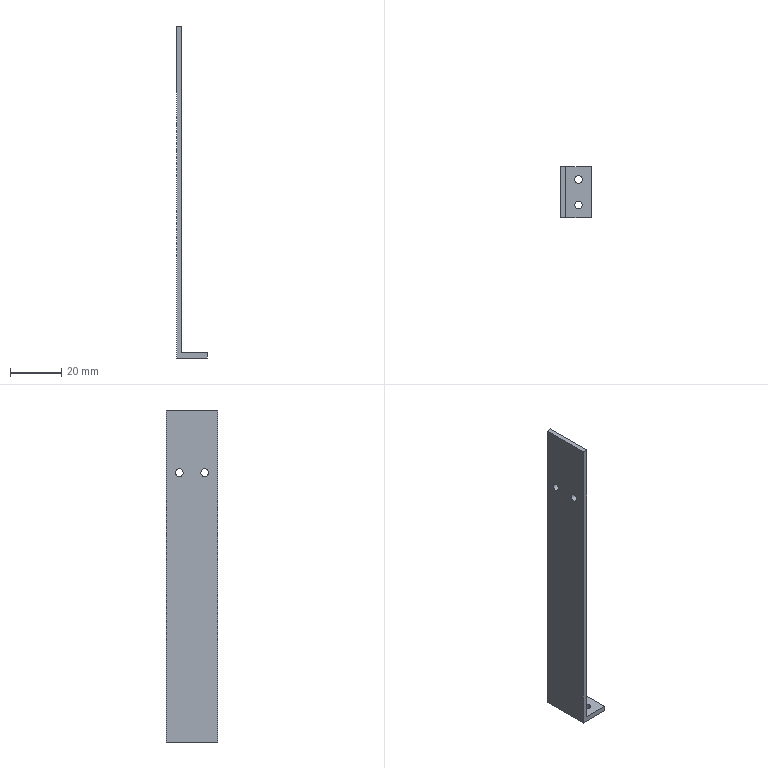Part | SolidWorks | features Cut 2, Extrusion 1, ICE 1 | 1 solid | 16 faces | box 12 x 20 x 130 mm | volume 5543 mm3 | cylinder 8 | plane 8 | commonest cylinder face diameters 3 x8
STEP:
#1=CARTESIAN_POINT('',(10.,-5.,106.942));
#2=VERTEX_POINT('',#1);
#3=CARTESIAN_POINT('',(10.,-5.,103.942));
#4=VERTEX_POINT('',#3);
#5=CARTESIAN_POINT('',(10.,-5.,105.442));
#6=DIRECTION('',(1.,0.,0.));
#7=DIRECTION('',(0.,0.,-1.));
#8=AXIS2_PLACEMENT_3D('',#5,#6,#7);
#9=CIRCLE('',#8,1.5);
#10=EDGE_CURVE('',#2,#4,#9,.T.);
#11=ORIENTED_EDGE('',*,*,#10,.F.);
#12=CARTESIAN_POINT('',(12.,-5.,106.942));
#13=VERTEX_POINT('',#12);
#14=CARTESIAN_POINT('',(-33.,-5.,106.942));
#15=DIRECTION('',(1.,0.,0.));
#16=VECTOR('',#15,1000.);
#17=LINE('',#14,#16);
#18=EDGE_CURVE('',#2,#13,#17,.T.);
#19=ORIENTED_EDGE('',*,*,#18,.T.);
#20=CARTESIAN_POINT('',(12.,-5.,103.942));
#21=VERTEX_POINT('',#20);
#22=CARTESIAN_POINT('',(12.,-5.,105.442));
#23=DIRECTION('',(1.,0.,0.));
#24=DIRECTION('',(0.,0.,-1.));
#25=AXIS2_PLACEMENT_3D('',#22,#23,#24);
#26=CIRCLE('',#25,1.5);
#27=EDGE_CURVE('',#13,#21,#26,.T.);
#28=ORIENTED_EDGE('',*,*,#27,.T.);
#29=CARTESIAN_POINT('',(-33.,-5.,103.942));
#30=DIRECTION('',(1.,0.,0.));
#31=VECTOR('',#30,1000.);
#32=LINE('',#29,#31);
#33=EDGE_CURVE('',#4,#21,#32,.T.);
#34=ORIENTED_EDGE('',*,*,#33,.F.);
#35=EDGE_LOOP('',(#11,#19,#28,#34));
#36=FACE_OUTER_BOUND('',#35,.T.);
#37=CARTESIAN_POINT('',(-33.,-5.,105.442));
#38=DIRECTION('',(1.,0.,0.));
#39=DIRECTION('',(0.,0.,-1.));
#40=AXIS2_PLACEMENT_3D('',#37,#38,#39);
#41=CYLINDRICAL_SURFACE('',#40,1.5);
#42=ADVANCED_FACE('',(#36),#41,.F.);
#43=CARTESIAN_POINT('',(10.,5.,106.942));
#44=VERTEX_POINT('',#43);
#45=CARTESIAN_POINT('',(10.,5.,103.942));
#46=VERTEX_POINT('',#45);
#47=CARTESIAN_POINT('',(10.,5.,105.442));
#48=DIRECTION('',(1.,0.,0.));
#49=DIRECTION('',(0.,0.,-1.));
#50=AXIS2_PLACEMENT_3D('',#47,#48,#49);
#51=CIRCLE('',#50,1.5);
#52=EDGE_CURVE('',#44,#46,#51,.T.);
#53=ORIENTED_EDGE('',*,*,#52,.F.);
#54=CARTESIAN_POINT('',(12.,5.,106.942));
#55=VERTEX_POINT('',#54);
#56=CARTESIAN_POINT('',(-33.,5.,106.942));
#57=DIRECTION('',(1.,0.,0.));
#58=VECTOR('',#57,1000.);
#59=LINE('',#56,#58);
#60=EDGE_CURVE('',#44,#55,#59,.T.);
#61=ORIENTED_EDGE('',*,*,#60,.T.);
#62=CARTESIAN_POINT('',(12.,5.,103.942));
#63=VERTEX_POINT('',#62);
#64=CARTESIAN_POINT('',(12.,5.,105.442));
#65=DIRECTION('',(1.,0.,0.));
#66=DIRECTION('',(0.,0.,1.));
#67=AXIS2_PLACEMENT_3D('',#64,#65,#66);
#68=CIRCLE('',#67,1.5);
#69=EDGE_CURVE('',#55,#63,#68,.T.);
#70=ORIENTED_EDGE('',*,*,#69,.T.);
#71=CARTESIAN_POINT('',(-33.,5.,103.942));
#72=DIRECTION('',(1.,0.,0.));
#73=VECTOR('',#72,1000.);
#74=LINE('',#71,#73);
#75=EDGE_CURVE('',#46,#63,#74,.T.);
#76=ORIENTED_EDGE('',*,*,#75,.F.);
#77=EDGE_LOOP('',(#53,#61,#70,#76));
#78=FACE_OUTER_BOUND('',#77,.T.);
#79=CARTESIAN_POINT('',(-33.,5.,105.442));
#80=DIRECTION('',(1.,0.,0.));
#81=DIRECTION('',(0.,0.,-1.));
#82=AXIS2_PLACEMENT_3D('',#79,#80,#81);
#83=CYLINDRICAL_SURFACE('',#82,1.5);
#84=ADVANCED_FACE('',(#78),#83,.F.);
#85=CARTESIAN_POINT('',(15.5,5.,0.));
#86=VERTEX_POINT('',#85);
#87=CARTESIAN_POINT('',(18.5,5.,0.));
#88=VERTEX_POINT('',#87);
#89=CARTESIAN_POINT('',(17.,5.,0.));
#90=DIRECTION('',(0.,0.,1.));
#91=DIRECTION('',(1.,0.,0.));
#92=AXIS2_PLACEMENT_3D('',#89,#90,#91);
#93=CIRCLE('',#92,1.5);
#94=EDGE_CURVE('',#86,#88,#93,.T.);
#95=ORIENTED_EDGE('',*,*,#94,.F.);
#96=CARTESIAN_POINT('',(15.5,5.,2.));
#97=VERTEX_POINT('',#96);
#98=CARTESIAN_POINT('',(15.5,5.,-4.));
#99=DIRECTION('',(0.,0.,1.));
#100=VECTOR('',#99,1000.);
#101=LINE('',#98,#100);
#102=EDGE_CURVE('',#86,#97,#101,.T.);
#103=ORIENTED_EDGE('',*,*,#102,.T.);
#104=CARTESIAN_POINT('',(18.5,5.,2.));
#105=VERTEX_POINT('',#104);
#106=CARTESIAN_POINT('',(17.,5.,2.));
#107=DIRECTION('',(0.,0.,1.));
#108=DIRECTION('',(1.,0.,0.));
#109=AXIS2_PLACEMENT_3D('',#106,#107,#108);
#110=CIRCLE('',#109,1.5);
#111=EDGE_CURVE('',#97,#105,#110,.T.);
#112=ORIENTED_EDGE('',*,*,#111,.T.);
#113=CARTESIAN_POINT('',(18.5,5.,-4.));
#114=DIRECTION('',(0.,0.,1.));
#115=VECTOR('',#114,1000.);
#116=LINE('',#113,#115);
#117=EDGE_CURVE('',#88,#105,#116,.T.);
#118=ORIENTED_EDGE('',*,*,#117,.F.);
#119=EDGE_LOOP('',(#95,#103,#112,#118));
#120=FACE_OUTER_BOUND('',#119,.T.);
#121=CARTESIAN_POINT('',(17.,5.,-4.));
#122=DIRECTION('',(0.,0.,1.));
#123=DIRECTION('',(1.,0.,0.));
#124=AXIS2_PLACEMENT_3D('',#121,#122,#123);
#125=CYLINDRICAL_SURFACE('',#124,1.5);
#126=ADVANCED_FACE('',(#120),#125,.F.);
#127=CARTESIAN_POINT('',(15.5,-5.,0.));
#128=VERTEX_POINT('',#127);
#129=CARTESIAN_POINT('',(18.5,-5.,0.));
#130=VERTEX_POINT('',#129);
#131=CARTESIAN_POINT('',(17.,-5.,0.));
#132=DIRECTION('',(0.,0.,1.));
#133=DIRECTION('',(1.,0.,0.));
#134=AXIS2_PLACEMENT_3D('',#131,#132,#133);
#135=CIRCLE('',#134,1.5);
#136=EDGE_CURVE('',#128,#130,#135,.T.);
#137=ORIENTED_EDGE('',*,*,#136,.F.);
#138=CARTESIAN_POINT('',(15.5,-5.,2.));
#139=VERTEX_POINT('',#138);
#140=CARTESIAN_POINT('',(15.5,-5.,-4.));
#141=DIRECTION('',(0.,0.,1.));
#142=VECTOR('',#141,1000.);
#143=LINE('',#140,#142);
#144=EDGE_CURVE('',#128,#139,#143,.T.);
#145=ORIENTED_EDGE('',*,*,#144,.T.);
#146=CARTESIAN_POINT('',(18.5,-5.,2.));
#147=VERTEX_POINT('',#146);
#148=CARTESIAN_POINT('',(17.,-5.,2.));
#149=DIRECTION('',(0.,0.,1.));
#150=DIRECTION('',(-1.,0.,0.));
#151=AXIS2_PLACEMENT_3D('',#148,#149,#150);
#152=CIRCLE('',#151,1.5);
#153=EDGE_CURVE('',#139,#147,#152,.T.);
#154=ORIENTED_EDGE('',*,*,#153,.T.);
#155=CARTESIAN_POINT('',(18.5,-5.,-4.));
#156=DIRECTION('',(0.,0.,1.));
#157=VECTOR('',#156,1000.);
#158=LINE('',#155,#157);
#159=EDGE_CURVE('',#130,#147,#158,.T.);
#160=ORIENTED_EDGE('',*,*,#159,.F.);
#161=EDGE_LOOP('',(#137,#145,#154,#160));
#162=FACE_OUTER_BOUND('',#161,.T.);
#163=CARTESIAN_POINT('',(17.,-5.,-4.));
#164=DIRECTION('',(0.,0.,1.));
#165=DIRECTION('',(1.,0.,0.));
#166=AXIS2_PLACEMENT_3D('',#163,#164,#165);
#167=CYLINDRICAL_SURFACE('',#166,1.5);
#168=ADVANCED_FACE('',(#162),#167,.F.);
#169=CARTESIAN_POINT('',(12.,-5.,105.442));
#170=DIRECTION('',(1.,0.,0.));
#171=DIRECTION('',(0.,0.,-1.));
#172=AXIS2_PLACEMENT_3D('',#169,#170,#171);
#173=CIRCLE('',#172,1.5);
#174=EDGE_CURVE('',#21,#13,#173,.T.);
#175=ORIENTED_EDGE('',*,*,#174,.F.);
#176=ORIENTED_EDGE('',*,*,#27,.F.);
#177=EDGE_LOOP('',(#175,#176));
#178=FACE_BOUND('',#177,.T.);
#179=CARTESIAN_POINT('',(12.,5.,105.442));
#180=DIRECTION('',(1.,0.,0.));
#181=DIRECTION('',(0.,0.,1.));
#182=AXIS2_PLACEMENT_3D('',#179,#180,#181);
#183=CIRCLE('',#182,1.5);
#184=EDGE_CURVE('',#63,#55,#183,.T.);
#185=ORIENTED_EDGE('',*,*,#184,.F.);
#186=ORIENTED_EDGE('',*,*,#69,.F.);
#187=EDGE_LOOP('',(#185,#186));
#188=FACE_BOUND('',#187,.T.);
#189=CARTESIAN_POINT('',(12.,10.,2.));
#190=VERTEX_POINT('',#189);
#191=CARTESIAN_POINT('',(12.,-10.,2.));
#192=VERTEX_POINT('',#191);
#193=CARTESIAN_POINT('',(12.,-10.,2.));
#194=DIRECTION('',(0.,-1.,0.));
#195=VECTOR('',#194,1000.);
#196=LINE('',#193,#195);
#197=EDGE_CURVE('',#190,#192,#196,.T.);
#198=ORIENTED_EDGE('',*,*,#197,.F.);
#199=CARTESIAN_POINT('',(12.,10.,130.));
#200=VERTEX_POINT('',#199);
#201=CARTESIAN_POINT('',(12.,10.,130.));
#202=DIRECTION('',(0.,0.,-1.));
#203=VECTOR('',#202,1000.);
#204=LINE('',#201,#203);
#205=EDGE_CURVE('',#200,#190,#204,.T.);
#206=ORIENTED_EDGE('',*,*,#205,.F.);
#207=CARTESIAN_POINT('',(12.,-10.,130.));
#208=VERTEX_POINT('',#207);
#209=CARTESIAN_POINT('',(12.,10.,130.));
#210=DIRECTION('',(0.,1.,0.));
#211=VECTOR('',#210,1000.);
#212=LINE('',#209,#211);
#213=EDGE_CURVE('',#208,#200,#212,.T.);
#214=ORIENTED_EDGE('',*,*,#213,.F.);
#215=CARTESIAN_POINT('',(12.,-10.,130.));
#216=DIRECTION('',(0.,0.,-1.));
#217=VECTOR('',#216,1000.);
#218=LINE('',#215,#217);
#219=EDGE_CURVE('',#208,#192,#218,.T.);
#220=ORIENTED_EDGE('',*,*,#219,.T.);
#221=EDGE_LOOP('',(#198,#206,#214,#220));
#222=FACE_OUTER_BOUND('',#221,.T.);
#223=CARTESIAN_POINT('',(12.,10.,130.));
#224=DIRECTION('',(-1.,0.,0.));
#225=DIRECTION('',(0.,0.,1.));
#226=AXIS2_PLACEMENT_3D('',#223,#224,#225);
#227=PLANE('',#226);
#228=ADVANCED_FACE('',(#178,#188,#222),#227,.F.);
#229=CARTESIAN_POINT('',(22.,10.,0.));
#230=VERTEX_POINT('',#229);
#231=CARTESIAN_POINT('',(10.,10.,0.));
#232=VERTEX_POINT('',#231);
#233=CARTESIAN_POINT('',(10.,10.,0.));
#234=DIRECTION('',(-1.,0.,0.));
#235=VECTOR('',#234,1000.);
#236=LINE('',#233,#235);
#237=EDGE_CURVE('',#230,#232,#236,.T.);
#238=ORIENTED_EDGE('',*,*,#237,.T.);
#239=CARTESIAN_POINT('',(10.,10.,130.));
#240=VERTEX_POINT('',#239);
#241=CARTESIAN_POINT('',(10.,10.,130.));
#242=DIRECTION('',(0.,0.,-1.));
#243=VECTOR('',#242,1000.);
#244=LINE('',#241,#243);
#245=EDGE_CURVE('',#240,#232,#244,.T.);
#246=ORIENTED_EDGE('',*,*,#245,.F.);
#247=CARTESIAN_POINT('',(10.,10.,130.));
#248=DIRECTION('',(-1.,0.,0.));
#249=VECTOR('',#248,1000.);
#250=LINE('',#247,#249);
#251=EDGE_CURVE('',#200,#240,#250,.T.);
#252=ORIENTED_EDGE('',*,*,#251,.F.);
#253=ORIENTED_EDGE('',*,*,#205,.T.);
#254=CARTESIAN_POINT('',(22.,10.,2.));
#255=VERTEX_POINT('',#254);
#256=CARTESIAN_POINT('',(12.,10.,2.));
#257=DIRECTION('',(-1.,0.,0.));
#258=VECTOR('',#257,1000.);
#259=LINE('',#256,#258);
#260=EDGE_CURVE('',#255,#190,#259,.T.);
#261=ORIENTED_EDGE('',*,*,#260,.F.);
#262=CARTESIAN_POINT('',(22.,10.,2.));
#263=DIRECTION('',(0.,0.,-1.));
#264=VECTOR('',#263,1000.);
#265=LINE('',#262,#264);
#266=EDGE_CURVE('',#255,#230,#265,.T.);
#267=ORIENTED_EDGE('',*,*,#266,.T.);
#268=EDGE_LOOP('',(#238,#246,#252,#253,#261,#267));
#269=FACE_OUTER_BOUND('',#268,.T.);
#270=CARTESIAN_POINT('',(10.,10.,130.));
#271=DIRECTION('',(0.,-1.,0.));
#272=DIRECTION('',(1.,0.,0.));
#273=AXIS2_PLACEMENT_3D('',#270,#271,#272);
#274=PLANE('',#273);
#275=ADVANCED_FACE('',(#269),#274,.F.);
#276=CARTESIAN_POINT('',(10.,-5.,105.442));
#277=DIRECTION('',(1.,0.,0.));
#278=DIRECTION('',(0.,0.,-1.));
#279=AXIS2_PLACEMENT_3D('',#276,#277,#278);
#280=CIRCLE('',#279,1.5);
#281=EDGE_CURVE('',#4,#2,#280,.T.);
#282=ORIENTED_EDGE('',*,*,#281,.T.);
#283=ORIENTED_EDGE('',*,*,#10,.T.);
#284=EDGE_LOOP('',(#282,#283));
#285=FACE_BOUND('',#284,.T.);
#286=CARTESIAN_POINT('',(10.,5.,105.442));
#287=DIRECTION('',(1.,0.,0.));
#288=DIRECTION('',(0.,0.,-1.));
#289=AXIS2_PLACEMENT_3D('',#286,#287,#288);
#290=CIRCLE('',#289,1.5);
#291=EDGE_CURVE('',#46,#44,#290,.T.);
#292=ORIENTED_EDGE('',*,*,#291,.T.);
#293=ORIENTED_EDGE('',*,*,#52,.T.);
#294=EDGE_LOOP('',(#292,#293));
#295=FACE_BOUND('',#294,.T.);
#296=CARTESIAN_POINT('',(10.,-10.,0.));
#297=VERTEX_POINT('',#296);
#298=CARTESIAN_POINT('',(10.,10.,0.));
#299=DIRECTION('',(0.,-1.,0.));
#300=VECTOR('',#299,1000.);
#301=LINE('',#298,#300);
#302=EDGE_CURVE('',#232,#297,#301,.T.);
#303=ORIENTED_EDGE('',*,*,#302,.T.);
#304=CARTESIAN_POINT('',(10.,-10.,130.));
#305=VERTEX_POINT('',#304);
#306=CARTESIAN_POINT('',(10.,-10.,130.));
#307=DIRECTION('',(0.,0.,-1.));
#308=VECTOR('',#307,1000.);
#309=LINE('',#306,#308);
#310=EDGE_CURVE('',#305,#297,#309,.T.);
#311=ORIENTED_EDGE('',*,*,#310,.F.);
#312=CARTESIAN_POINT('',(10.,10.,130.));
#313=DIRECTION('',(0.,-1.,0.));
#314=VECTOR('',#313,1000.);
#315=LINE('',#312,#314);
#316=EDGE_CURVE('',#240,#305,#315,.T.);
#317=ORIENTED_EDGE('',*,*,#316,.F.);
#318=ORIENTED_EDGE('',*,*,#245,.T.);
#319=EDGE_LOOP('',(#303,#311,#317,#318));
#320=FACE_OUTER_BOUND('',#319,.T.);
#321=CARTESIAN_POINT('',(10.,10.,130.));
#322=DIRECTION('',(1.,0.,0.));
#323=DIRECTION('',(0.,0.,-1.));
#324=AXIS2_PLACEMENT_3D('',#321,#322,#323);
#325=PLANE('',#324);
#326=ADVANCED_FACE('',(#285,#295,#320),#325,.F.);
#327=CARTESIAN_POINT('',(22.,-10.,0.));
#328=VERTEX_POINT('',#327);
#329=CARTESIAN_POINT('',(10.,-10.,0.));
#330=DIRECTION('',(1.,0.,0.));
#331=VECTOR('',#330,1000.);
#332=LINE('',#329,#331);
#333=EDGE_CURVE('',#297,#328,#332,.T.);
#334=ORIENTED_EDGE('',*,*,#333,.T.);
#335=CARTESIAN_POINT('',(22.,-10.,2.));
#336=VERTEX_POINT('',#335);
#337=CARTESIAN_POINT('',(22.,-10.,2.));
#338=DIRECTION('',(0.,0.,-1.));
#339=VECTOR('',#338,1000.);
#340=LINE('',#337,#339);
#341=EDGE_CURVE('',#336,#328,#340,.T.);
#342=ORIENTED_EDGE('',*,*,#341,.F.);
#343=CARTESIAN_POINT('',(22.,-10.,2.));
#344=DIRECTION('',(1.,0.,0.));
#345=VECTOR('',#344,1000.);
#346=LINE('',#343,#345);
#347=EDGE_CURVE('',#192,#336,#346,.T.);
#348=ORIENTED_EDGE('',*,*,#347,.F.);
#349=ORIENTED_EDGE('',*,*,#219,.F.);
#350=CARTESIAN_POINT('',(10.,-10.,130.));
#351=DIRECTION('',(1.,0.,0.));
#352=VECTOR('',#351,1000.);
#353=LINE('',#350,#352);
#354=EDGE_CURVE('',#305,#208,#353,.T.);
#355=ORIENTED_EDGE('',*,*,#354,.F.);
#356=ORIENTED_EDGE('',*,*,#310,.T.);
#357=EDGE_LOOP('',(#334,#342,#348,#349,#355,#356));
#358=FACE_OUTER_BOUND('',#357,.T.);
#359=CARTESIAN_POINT('',(10.,-10.,130.));
#360=DIRECTION('',(0.,1.,0.));
#361=DIRECTION('',(0.,0.,1.));
#362=AXIS2_PLACEMENT_3D('',#359,#360,#361);
#363=PLANE('',#362);
#364=ADVANCED_FACE('',(#358),#363,.F.);
#365=ORIENTED_EDGE('',*,*,#213,.T.);
#366=ORIENTED_EDGE('',*,*,#251,.T.);
#367=ORIENTED_EDGE('',*,*,#316,.T.);
#368=ORIENTED_EDGE('',*,*,#354,.T.);
#369=EDGE_LOOP('',(#365,#366,#367,#368));
#370=FACE_OUTER_BOUND('',#369,.T.);
#371=CARTESIAN_POINT('',(0.,0.,130.));
#372=DIRECTION('',(0.,0.,1.));
#373=DIRECTION('',(1.,0.,0.));
#374=AXIS2_PLACEMENT_3D('',#371,#372,#373);
#375=PLANE('',#374);
#376=ADVANCED_FACE('',(#370),#375,.T.);
#377=CARTESIAN_POINT('',(17.,5.,0.));
#378=DIRECTION('',(0.,0.,1.));
#379=DIRECTION('',(1.,0.,0.));
#380=AXIS2_PLACEMENT_3D('',#377,#378,#379);
#381=CIRCLE('',#380,1.5);
#382=EDGE_CURVE('',#88,#86,#381,.T.);
#383=ORIENTED_EDGE('',*,*,#382,.T.);
#384=ORIENTED_EDGE('',*,*,#94,.T.);
#385=EDGE_LOOP('',(#383,#384));
#386=FACE_BOUND('',#385,.T.);
#387=CARTESIAN_POINT('',(17.,-5.,0.));
#388=DIRECTION('',(0.,0.,1.));
#389=DIRECTION('',(1.,0.,0.));
#390=AXIS2_PLACEMENT_3D('',#387,#388,#389);
#391=CIRCLE('',#390,1.5);
#392=EDGE_CURVE('',#130,#128,#391,.T.);
#393=ORIENTED_EDGE('',*,*,#392,.T.);
#394=ORIENTED_EDGE('',*,*,#136,.T.);
#395=EDGE_LOOP('',(#393,#394));
#396=FACE_BOUND('',#395,.T.);
#397=ORIENTED_EDGE('',*,*,#237,.F.);
#398=CARTESIAN_POINT('',(22.,10.,0.));
#399=DIRECTION('',(0.,1.,0.));
#400=VECTOR('',#399,1000.);
#401=LINE('',#398,#400);
#402=EDGE_CURVE('',#328,#230,#401,.T.);
#403=ORIENTED_EDGE('',*,*,#402,.F.);
#404=ORIENTED_EDGE('',*,*,#333,.F.);
#405=ORIENTED_EDGE('',*,*,#302,.F.);
#406=EDGE_LOOP('',(#397,#403,#404,#405));
#407=FACE_OUTER_BOUND('',#406,.T.);
#408=CARTESIAN_POINT('',(0.,0.,0.));
#409=DIRECTION('',(0.,0.,1.));
#410=DIRECTION('',(1.,0.,0.));
#411=AXIS2_PLACEMENT_3D('',#408,#409,#410);
#412=PLANE('',#411);
#413=ADVANCED_FACE('',(#386,#396,#407),#412,.F.);
#414=ORIENTED_EDGE('',*,*,#402,.T.);
#415=ORIENTED_EDGE('',*,*,#266,.F.);
#416=CARTESIAN_POINT('',(22.,10.,2.));
#417=DIRECTION('',(0.,1.,0.));
#418=VECTOR('',#417,1000.);
#419=LINE('',#416,#418);
#420=EDGE_CURVE('',#336,#255,#419,.T.);
#421=ORIENTED_EDGE('',*,*,#420,.F.);
#422=ORIENTED_EDGE('',*,*,#341,.T.);
#423=EDGE_LOOP('',(#414,#415,#421,#422));
#424=FACE_OUTER_BOUND('',#423,.T.);
#425=CARTESIAN_POINT('',(22.,10.,2.));
#426=DIRECTION('',(-1.,0.,0.));
#427=DIRECTION('',(0.,-1.,0.));
#428=AXIS2_PLACEMENT_3D('',#425,#426,#427);
#429=PLANE('',#428);
#430=ADVANCED_FACE('',(#424),#429,.F.);
#431=CARTESIAN_POINT('',(17.,5.,2.));
#432=DIRECTION('',(0.,0.,1.));
#433=DIRECTION('',(1.,0.,0.));
#434=AXIS2_PLACEMENT_3D('',#431,#432,#433);
#435=CIRCLE('',#434,1.5);
#436=EDGE_CURVE('',#105,#97,#435,.T.);
#437=ORIENTED_EDGE('',*,*,#436,.F.);
#438=ORIENTED_EDGE('',*,*,#111,.F.);
#439=EDGE_LOOP('',(#437,#438));
#440=FACE_BOUND('',#439,.T.);
#441=CARTESIAN_POINT('',(17.,-5.,2.));
#442=DIRECTION('',(0.,0.,1.));
#443=DIRECTION('',(-1.,0.,0.));
#444=AXIS2_PLACEMENT_3D('',#441,#442,#443);
#445=CIRCLE('',#444,1.5);
#446=EDGE_CURVE('',#147,#139,#445,.T.);
#447=ORIENTED_EDGE('',*,*,#446,.F.);
#448=ORIENTED_EDGE('',*,*,#153,.F.);
#449=EDGE_LOOP('',(#447,#448));
#450=FACE_BOUND('',#449,.T.);
#451=ORIENTED_EDGE('',*,*,#347,.T.);
#452=ORIENTED_EDGE('',*,*,#420,.T.);
#453=ORIENTED_EDGE('',*,*,#260,.T.);
#454=ORIENTED_EDGE('',*,*,#197,.T.);
#455=EDGE_LOOP('',(#451,#452,#453,#454));
#456=FACE_OUTER_BOUND('',#455,.T.);
#457=CARTESIAN_POINT('',(0.,0.,2.));
#458=DIRECTION('',(0.,0.,-1.));
#459=DIRECTION('',(-1.,0.,0.));
#460=AXIS2_PLACEMENT_3D('',#457,#458,#459);
#461=PLANE('',#460);
#462=ADVANCED_FACE('',(#440,#450,#456),#461,.F.);
#463=ORIENTED_EDGE('',*,*,#144,.F.);
#464=ORIENTED_EDGE('',*,*,#392,.F.);
#465=ORIENTED_EDGE('',*,*,#159,.T.);
#466=ORIENTED_EDGE('',*,*,#446,.T.);
#467=EDGE_LOOP('',(#463,#464,#465,#466));
#468=FACE_OUTER_BOUND('',#467,.T.);
#469=CARTESIAN_POINT('',(17.,-5.,-4.));
#470=DIRECTION('',(0.,0.,1.));
#471=DIRECTION('',(1.,0.,0.));
#472=AXIS2_PLACEMENT_3D('',#469,#470,#471);
#473=CYLINDRICAL_SURFACE('',#472,1.5);
#474=ADVANCED_FACE('',(#468),#473,.F.);
#475=ORIENTED_EDGE('',*,*,#102,.F.);
#476=ORIENTED_EDGE('',*,*,#382,.F.);
#477=ORIENTED_EDGE('',*,*,#117,.T.);
#478=ORIENTED_EDGE('',*,*,#436,.T.);
#479=EDGE_LOOP('',(#475,#476,#477,#478));
#480=FACE_OUTER_BOUND('',#479,.T.);
#481=CARTESIAN_POINT('',(17.,5.,-4.));
#482=DIRECTION('',(0.,0.,1.));
#483=DIRECTION('',(1.,0.,0.));
#484=AXIS2_PLACEMENT_3D('',#481,#482,#483);
#485=CYLINDRICAL_SURFACE('',#484,1.5);
#486=ADVANCED_FACE('',(#480),#485,.F.);
#487=ORIENTED_EDGE('',*,*,#60,.F.);
#488=ORIENTED_EDGE('',*,*,#291,.F.);
#489=ORIENTED_EDGE('',*,*,#75,.T.);
#490=ORIENTED_EDGE('',*,*,#184,.T.);
#491=EDGE_LOOP('',(#487,#488,#489,#490));
#492=FACE_OUTER_BOUND('',#491,.T.);
#493=CARTESIAN_POINT('',(-33.,5.,105.442));
#494=DIRECTION('',(1.,0.,0.));
#495=DIRECTION('',(0.,0.,-1.));
#496=AXIS2_PLACEMENT_3D('',#493,#494,#495);
#497=CYLINDRICAL_SURFACE('',#496,1.5);
#498=ADVANCED_FACE('',(#492),#497,.F.);
#499=ORIENTED_EDGE('',*,*,#18,.F.);
#500=ORIENTED_EDGE('',*,*,#281,.F.);
#501=ORIENTED_EDGE('',*,*,#33,.T.);
#502=ORIENTED_EDGE('',*,*,#174,.T.);
#503=EDGE_LOOP('',(#499,#500,#501,#502));
#504=FACE_OUTER_BOUND('',#503,.T.);
#505=CARTESIAN_POINT('',(-33.,-5.,105.442));
#506=DIRECTION('',(1.,0.,0.));
#507=DIRECTION('',(0.,0.,-1.));
#508=AXIS2_PLACEMENT_3D('',#505,#506,#507);
#509=CYLINDRICAL_SURFACE('',#508,1.5);
#510=ADVANCED_FACE('',(#504),#509,.F.);
#511=CLOSED_SHELL('',(#42,#84,#126,#168,#228,#275,#326,#364,#376,#413,#430,#462,#474,#486,#498,#510));
#512=MANIFOLD_SOLID_BREP('',#511);
#513=CARTESIAN_POINT('',(0.,0.,0.));
#514=DIRECTION('',(0.,0.,1.));
#515=DIRECTION('',(1.,0.,0.));
#516=AXIS2_PLACEMENT_3D('',#513,#514,#515);
#517=(LENGTH_UNIT()NAMED_UNIT(*)SI_UNIT(.MILLI.,.METRE.));
#518=UNCERTAINTY_MEASURE_WITH_UNIT(LENGTH_MEASURE(0.00001),#517,'','');
#519=(NAMED_UNIT(*)PLANE_ANGLE_UNIT()SI_UNIT($,.RADIAN.));
#520=(NAMED_UNIT(*)SI_UNIT($,.STERADIAN.)SOLID_ANGLE_UNIT());
#521=(GEOMETRIC_REPRESENTATION_CONTEXT(3)GLOBAL_UNCERTAINTY_ASSIGNED_CONTEXT((#518))GLOBAL_UNIT_ASSIGNED_CONTEXT((#517,#519,#520))REPRESENTATION_CONTEXT('',''));
#522=ADVANCED_BREP_SHAPE_REPRESENTATION('',(#512,#516),#521);